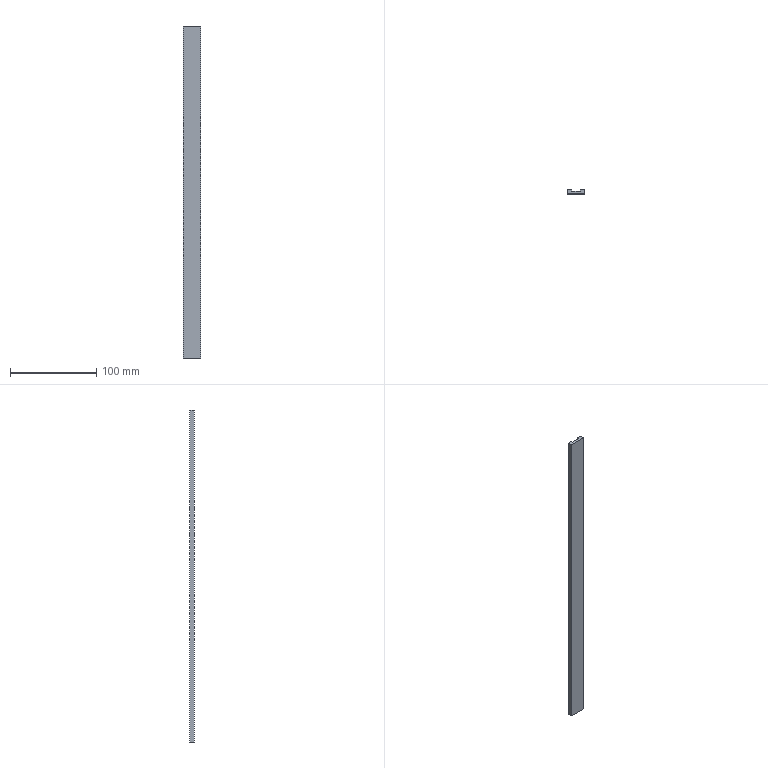Part | SolidWorks | features Extrusion 1 | 1 solid | 10 faces | box 20 x 5 x 385 mm | volume 30800 mm3 | plane 10
STEP:
#1=CARTESIAN_POINT('',(0.,5.,0.));
#2=VERTEX_POINT('',#1);
#3=CARTESIAN_POINT('',(0.,0.,0.));
#4=VERTEX_POINT('',#3);
#5=CARTESIAN_POINT('',(0.,0.,0.));
#6=DIRECTION('',(0.,-1.,0.));
#7=VECTOR('',#6,1000.);
#8=LINE('',#5,#7);
#9=EDGE_CURVE('',#2,#4,#8,.T.);
#10=ORIENTED_EDGE('',*,*,#9,.T.);
#11=CARTESIAN_POINT('',(0.,0.,385.));
#12=VERTEX_POINT('',#11);
#13=CARTESIAN_POINT('',(0.,0.,385.));
#14=DIRECTION('',(0.,0.,-1.));
#15=VECTOR('',#14,1000.);
#16=LINE('',#13,#15);
#17=EDGE_CURVE('',#12,#4,#16,.T.);
#18=ORIENTED_EDGE('',*,*,#17,.F.);
#19=CARTESIAN_POINT('',(0.,5.,385.));
#20=VERTEX_POINT('',#19);
#21=CARTESIAN_POINT('',(0.,0.,385.));
#22=DIRECTION('',(0.,-1.,0.));
#23=VECTOR('',#22,1000.);
#24=LINE('',#21,#23);
#25=EDGE_CURVE('',#20,#12,#24,.T.);
#26=ORIENTED_EDGE('',*,*,#25,.F.);
#27=CARTESIAN_POINT('',(0.,5.,385.));
#28=DIRECTION('',(0.,0.,-1.));
#29=VECTOR('',#28,1000.);
#30=LINE('',#27,#29);
#31=EDGE_CURVE('',#20,#2,#30,.T.);
#32=ORIENTED_EDGE('',*,*,#31,.T.);
#33=EDGE_LOOP('',(#10,#18,#26,#32));
#34=FACE_OUTER_BOUND('',#33,.T.);
#35=CARTESIAN_POINT('',(0.,0.,385.));
#36=DIRECTION('',(1.,0.,0.));
#37=DIRECTION('',(0.,0.,-1.));
#38=AXIS2_PLACEMENT_3D('',#35,#36,#37);
#39=PLANE('',#38);
#40=ADVANCED_FACE('',(#34),#39,.F.);
#41=CARTESIAN_POINT('',(20.,0.,0.));
#42=VERTEX_POINT('',#41);
#43=CARTESIAN_POINT('',(0.,0.,0.));
#44=DIRECTION('',(1.,0.,0.));
#45=VECTOR('',#44,1000.);
#46=LINE('',#43,#45);
#47=EDGE_CURVE('',#4,#42,#46,.T.);
#48=ORIENTED_EDGE('',*,*,#47,.T.);
#49=CARTESIAN_POINT('',(20.,0.,385.));
#50=VERTEX_POINT('',#49);
#51=CARTESIAN_POINT('',(20.,0.,385.));
#52=DIRECTION('',(0.,0.,-1.));
#53=VECTOR('',#52,1000.);
#54=LINE('',#51,#53);
#55=EDGE_CURVE('',#50,#42,#54,.T.);
#56=ORIENTED_EDGE('',*,*,#55,.F.);
#57=CARTESIAN_POINT('',(0.,0.,385.));
#58=DIRECTION('',(1.,0.,0.));
#59=VECTOR('',#58,1000.);
#60=LINE('',#57,#59);
#61=EDGE_CURVE('',#12,#50,#60,.T.);
#62=ORIENTED_EDGE('',*,*,#61,.F.);
#63=ORIENTED_EDGE('',*,*,#17,.T.);
#64=EDGE_LOOP('',(#48,#56,#62,#63));
#65=FACE_OUTER_BOUND('',#64,.T.);
#66=CARTESIAN_POINT('',(0.,0.,385.));
#67=DIRECTION('',(0.,1.,0.));
#68=DIRECTION('',(0.,0.,1.));
#69=AXIS2_PLACEMENT_3D('',#66,#67,#68);
#70=PLANE('',#69);
#71=ADVANCED_FACE('',(#65),#70,.F.);
#72=CARTESIAN_POINT('',(20.,5.,0.));
#73=VERTEX_POINT('',#72);
#74=CARTESIAN_POINT('',(20.,0.,0.));
#75=DIRECTION('',(0.,1.,0.));
#76=VECTOR('',#75,1000.);
#77=LINE('',#74,#76);
#78=EDGE_CURVE('',#42,#73,#77,.T.);
#79=ORIENTED_EDGE('',*,*,#78,.T.);
#80=CARTESIAN_POINT('',(20.,5.,385.));
#81=VERTEX_POINT('',#80);
#82=CARTESIAN_POINT('',(20.,5.,385.));
#83=DIRECTION('',(0.,0.,-1.));
#84=VECTOR('',#83,1000.);
#85=LINE('',#82,#84);
#86=EDGE_CURVE('',#81,#73,#85,.T.);
#87=ORIENTED_EDGE('',*,*,#86,.F.);
#88=CARTESIAN_POINT('',(20.,0.,385.));
#89=DIRECTION('',(0.,1.,0.));
#90=VECTOR('',#89,1000.);
#91=LINE('',#88,#90);
#92=EDGE_CURVE('',#50,#81,#91,.T.);
#93=ORIENTED_EDGE('',*,*,#92,.F.);
#94=ORIENTED_EDGE('',*,*,#55,.T.);
#95=EDGE_LOOP('',(#79,#87,#93,#94));
#96=FACE_OUTER_BOUND('',#95,.T.);
#97=CARTESIAN_POINT('',(20.,0.,385.));
#98=DIRECTION('',(-1.,0.,0.));
#99=DIRECTION('',(0.,0.,1.));
#100=AXIS2_PLACEMENT_3D('',#97,#98,#99);
#101=PLANE('',#100);
#102=ADVANCED_FACE('',(#96),#101,.F.);
#103=CARTESIAN_POINT('',(15.,5.,0.));
#104=VERTEX_POINT('',#103);
#105=CARTESIAN_POINT('',(15.,5.,0.));
#106=DIRECTION('',(-1.,0.,0.));
#107=VECTOR('',#106,1000.);
#108=LINE('',#105,#107);
#109=EDGE_CURVE('',#73,#104,#108,.T.);
#110=ORIENTED_EDGE('',*,*,#109,.T.);
#111=CARTESIAN_POINT('',(15.,5.,385.));
#112=VERTEX_POINT('',#111);
#113=CARTESIAN_POINT('',(15.,5.,385.));
#114=DIRECTION('',(0.,0.,-1.));
#115=VECTOR('',#114,1000.);
#116=LINE('',#113,#115);
#117=EDGE_CURVE('',#112,#104,#116,.T.);
#118=ORIENTED_EDGE('',*,*,#117,.F.);
#119=CARTESIAN_POINT('',(15.,5.,385.));
#120=DIRECTION('',(-1.,0.,0.));
#121=VECTOR('',#120,1000.);
#122=LINE('',#119,#121);
#123=EDGE_CURVE('',#81,#112,#122,.T.);
#124=ORIENTED_EDGE('',*,*,#123,.F.);
#125=ORIENTED_EDGE('',*,*,#86,.T.);
#126=EDGE_LOOP('',(#110,#118,#124,#125));
#127=FACE_OUTER_BOUND('',#126,.T.);
#128=CARTESIAN_POINT('',(15.,5.,385.));
#129=DIRECTION('',(0.,-1.,0.));
#130=DIRECTION('',(0.,0.,-1.));
#131=AXIS2_PLACEMENT_3D('',#128,#129,#130);
#132=PLANE('',#131);
#133=ADVANCED_FACE('',(#127),#132,.F.);
#134=CARTESIAN_POINT('',(15.,3.,0.));
#135=VERTEX_POINT('',#134);
#136=CARTESIAN_POINT('',(15.,3.,0.));
#137=DIRECTION('',(0.,-1.,0.));
#138=VECTOR('',#137,1000.);
#139=LINE('',#136,#138);
#140=EDGE_CURVE('',#104,#135,#139,.T.);
#141=ORIENTED_EDGE('',*,*,#140,.T.);
#142=CARTESIAN_POINT('',(15.,3.,385.));
#143=VERTEX_POINT('',#142);
#144=CARTESIAN_POINT('',(15.,3.,385.));
#145=DIRECTION('',(0.,0.,-1.));
#146=VECTOR('',#145,1000.);
#147=LINE('',#144,#146);
#148=EDGE_CURVE('',#143,#135,#147,.T.);
#149=ORIENTED_EDGE('',*,*,#148,.F.);
#150=CARTESIAN_POINT('',(15.,3.,385.));
#151=DIRECTION('',(0.,-1.,0.));
#152=VECTOR('',#151,1000.);
#153=LINE('',#150,#152);
#154=EDGE_CURVE('',#112,#143,#153,.T.);
#155=ORIENTED_EDGE('',*,*,#154,.F.);
#156=ORIENTED_EDGE('',*,*,#117,.T.);
#157=EDGE_LOOP('',(#141,#149,#155,#156));
#158=FACE_OUTER_BOUND('',#157,.T.);
#159=CARTESIAN_POINT('',(15.,3.,385.));
#160=DIRECTION('',(1.,0.,0.));
#161=DIRECTION('',(0.,0.,-1.));
#162=AXIS2_PLACEMENT_3D('',#159,#160,#161);
#163=PLANE('',#162);
#164=ADVANCED_FACE('',(#158),#163,.F.);
#165=CARTESIAN_POINT('',(5.,3.,0.));
#166=VERTEX_POINT('',#165);
#167=CARTESIAN_POINT('',(5.,3.,0.));
#168=DIRECTION('',(-1.,0.,0.));
#169=VECTOR('',#168,1000.);
#170=LINE('',#167,#169);
#171=EDGE_CURVE('',#135,#166,#170,.T.);
#172=ORIENTED_EDGE('',*,*,#171,.T.);
#173=CARTESIAN_POINT('',(5.,3.,385.));
#174=VERTEX_POINT('',#173);
#175=CARTESIAN_POINT('',(5.,3.,385.));
#176=DIRECTION('',(0.,0.,-1.));
#177=VECTOR('',#176,1000.);
#178=LINE('',#175,#177);
#179=EDGE_CURVE('',#174,#166,#178,.T.);
#180=ORIENTED_EDGE('',*,*,#179,.F.);
#181=CARTESIAN_POINT('',(5.,3.,385.));
#182=DIRECTION('',(-1.,0.,0.));
#183=VECTOR('',#182,1000.);
#184=LINE('',#181,#183);
#185=EDGE_CURVE('',#143,#174,#184,.T.);
#186=ORIENTED_EDGE('',*,*,#185,.F.);
#187=ORIENTED_EDGE('',*,*,#148,.T.);
#188=EDGE_LOOP('',(#172,#180,#186,#187));
#189=FACE_OUTER_BOUND('',#188,.T.);
#190=CARTESIAN_POINT('',(5.,3.,385.));
#191=DIRECTION('',(0.,-1.,0.));
#192=DIRECTION('',(0.,0.,-1.));
#193=AXIS2_PLACEMENT_3D('',#190,#191,#192);
#194=PLANE('',#193);
#195=ADVANCED_FACE('',(#189),#194,.F.);
#196=CARTESIAN_POINT('',(5.,5.,0.));
#197=VERTEX_POINT('',#196);
#198=CARTESIAN_POINT('',(5.,5.,0.));
#199=DIRECTION('',(0.,1.,0.));
#200=VECTOR('',#199,1000.);
#201=LINE('',#198,#200);
#202=EDGE_CURVE('',#166,#197,#201,.T.);
#203=ORIENTED_EDGE('',*,*,#202,.T.);
#204=CARTESIAN_POINT('',(5.,5.,385.));
#205=VERTEX_POINT('',#204);
#206=CARTESIAN_POINT('',(5.,5.,385.));
#207=DIRECTION('',(0.,0.,-1.));
#208=VECTOR('',#207,1000.);
#209=LINE('',#206,#208);
#210=EDGE_CURVE('',#205,#197,#209,.T.);
#211=ORIENTED_EDGE('',*,*,#210,.F.);
#212=CARTESIAN_POINT('',(5.,5.,385.));
#213=DIRECTION('',(0.,1.,0.));
#214=VECTOR('',#213,1000.);
#215=LINE('',#212,#214);
#216=EDGE_CURVE('',#174,#205,#215,.T.);
#217=ORIENTED_EDGE('',*,*,#216,.F.);
#218=ORIENTED_EDGE('',*,*,#179,.T.);
#219=EDGE_LOOP('',(#203,#211,#217,#218));
#220=FACE_OUTER_BOUND('',#219,.T.);
#221=CARTESIAN_POINT('',(5.,5.,385.));
#222=DIRECTION('',(-1.,0.,0.));
#223=DIRECTION('',(0.,0.,1.));
#224=AXIS2_PLACEMENT_3D('',#221,#222,#223);
#225=PLANE('',#224);
#226=ADVANCED_FACE('',(#220),#225,.F.);
#227=CARTESIAN_POINT('',(0.,5.,0.));
#228=DIRECTION('',(-1.,0.,0.));
#229=VECTOR('',#228,1000.);
#230=LINE('',#227,#229);
#231=EDGE_CURVE('',#197,#2,#230,.T.);
#232=ORIENTED_EDGE('',*,*,#231,.T.);
#233=ORIENTED_EDGE('',*,*,#31,.F.);
#234=CARTESIAN_POINT('',(0.,5.,385.));
#235=DIRECTION('',(-1.,0.,0.));
#236=VECTOR('',#235,1000.);
#237=LINE('',#234,#236);
#238=EDGE_CURVE('',#205,#20,#237,.T.);
#239=ORIENTED_EDGE('',*,*,#238,.F.);
#240=ORIENTED_EDGE('',*,*,#210,.T.);
#241=EDGE_LOOP('',(#232,#233,#239,#240));
#242=FACE_OUTER_BOUND('',#241,.T.);
#243=CARTESIAN_POINT('',(0.,5.,385.));
#244=DIRECTION('',(0.,-1.,0.));
#245=DIRECTION('',(0.,0.,-1.));
#246=AXIS2_PLACEMENT_3D('',#243,#244,#245);
#247=PLANE('',#246);
#248=ADVANCED_FACE('',(#242),#247,.F.);
#249=ORIENTED_EDGE('',*,*,#25,.T.);
#250=ORIENTED_EDGE('',*,*,#61,.T.);
#251=ORIENTED_EDGE('',*,*,#92,.T.);
#252=ORIENTED_EDGE('',*,*,#123,.T.);
#253=ORIENTED_EDGE('',*,*,#154,.T.);
#254=ORIENTED_EDGE('',*,*,#185,.T.);
#255=ORIENTED_EDGE('',*,*,#216,.T.);
#256=ORIENTED_EDGE('',*,*,#238,.T.);
#257=EDGE_LOOP('',(#249,#250,#251,#252,#253,#254,#255,#256));
#258=FACE_OUTER_BOUND('',#257,.T.);
#259=CARTESIAN_POINT('',(0.,0.,385.));
#260=DIRECTION('',(0.,0.,-1.));
#261=DIRECTION('',(-1.,0.,0.));
#262=AXIS2_PLACEMENT_3D('',#259,#260,#261);
#263=PLANE('',#262);
#264=ADVANCED_FACE('',(#258),#263,.F.);
#265=ORIENTED_EDGE('',*,*,#9,.F.);
#266=ORIENTED_EDGE('',*,*,#231,.F.);
#267=ORIENTED_EDGE('',*,*,#202,.F.);
#268=ORIENTED_EDGE('',*,*,#171,.F.);
#269=ORIENTED_EDGE('',*,*,#140,.F.);
#270=ORIENTED_EDGE('',*,*,#109,.F.);
#271=ORIENTED_EDGE('',*,*,#78,.F.);
#272=ORIENTED_EDGE('',*,*,#47,.F.);
#273=EDGE_LOOP('',(#265,#266,#267,#268,#269,#270,#271,#272));
#274=FACE_OUTER_BOUND('',#273,.T.);
#275=CARTESIAN_POINT('',(0.,0.,0.));
#276=DIRECTION('',(0.,0.,-1.));
#277=DIRECTION('',(-1.,0.,0.));
#278=AXIS2_PLACEMENT_3D('',#275,#276,#277);
#279=PLANE('',#278);
#280=ADVANCED_FACE('',(#274),#279,.T.);
#281=CLOSED_SHELL('',(#40,#71,#102,#133,#164,#195,#226,#248,#264,#280));
#282=MANIFOLD_SOLID_BREP('',#281);
#283=CARTESIAN_POINT('',(0.,0.,0.));
#284=DIRECTION('',(0.,0.,1.));
#285=DIRECTION('',(1.,0.,0.));
#286=AXIS2_PLACEMENT_3D('',#283,#284,#285);
#287=(LENGTH_UNIT()NAMED_UNIT(*)SI_UNIT(.MILLI.,.METRE.));
#288=UNCERTAINTY_MEASURE_WITH_UNIT(LENGTH_MEASURE(0.00001),#287,'','');
#289=(NAMED_UNIT(*)PLANE_ANGLE_UNIT()SI_UNIT($,.RADIAN.));
#290=(NAMED_UNIT(*)SI_UNIT($,.STERADIAN.)SOLID_ANGLE_UNIT());
#291=(GEOMETRIC_REPRESENTATION_CONTEXT(3)GLOBAL_UNCERTAINTY_ASSIGNED_CONTEXT((#288))GLOBAL_UNIT_ASSIGNED_CONTEXT((#287,#289,#290))REPRESENTATION_CONTEXT('',''));
#292=ADVANCED_BREP_SHAPE_REPRESENTATION('',(#282,#286),#291);